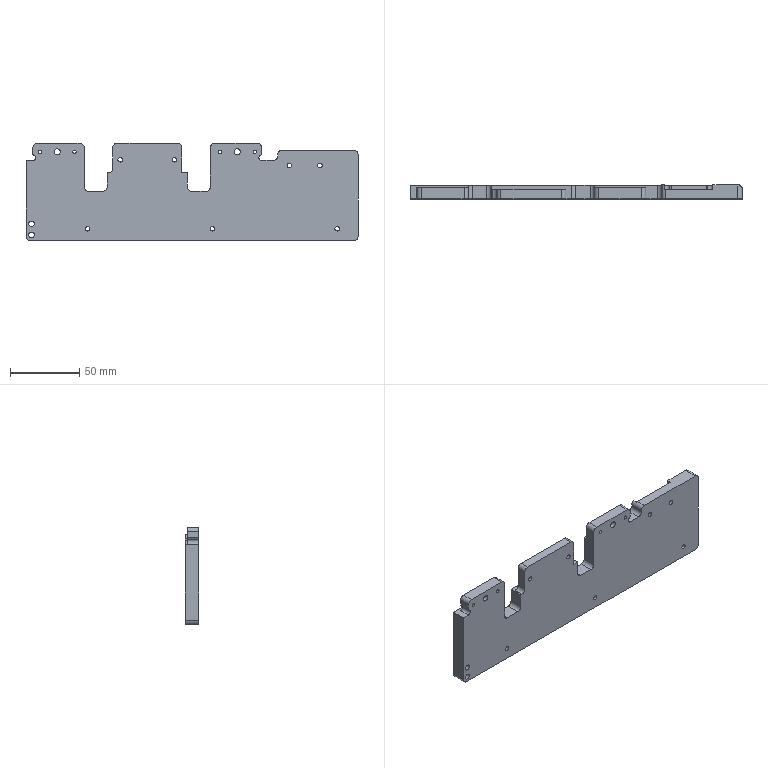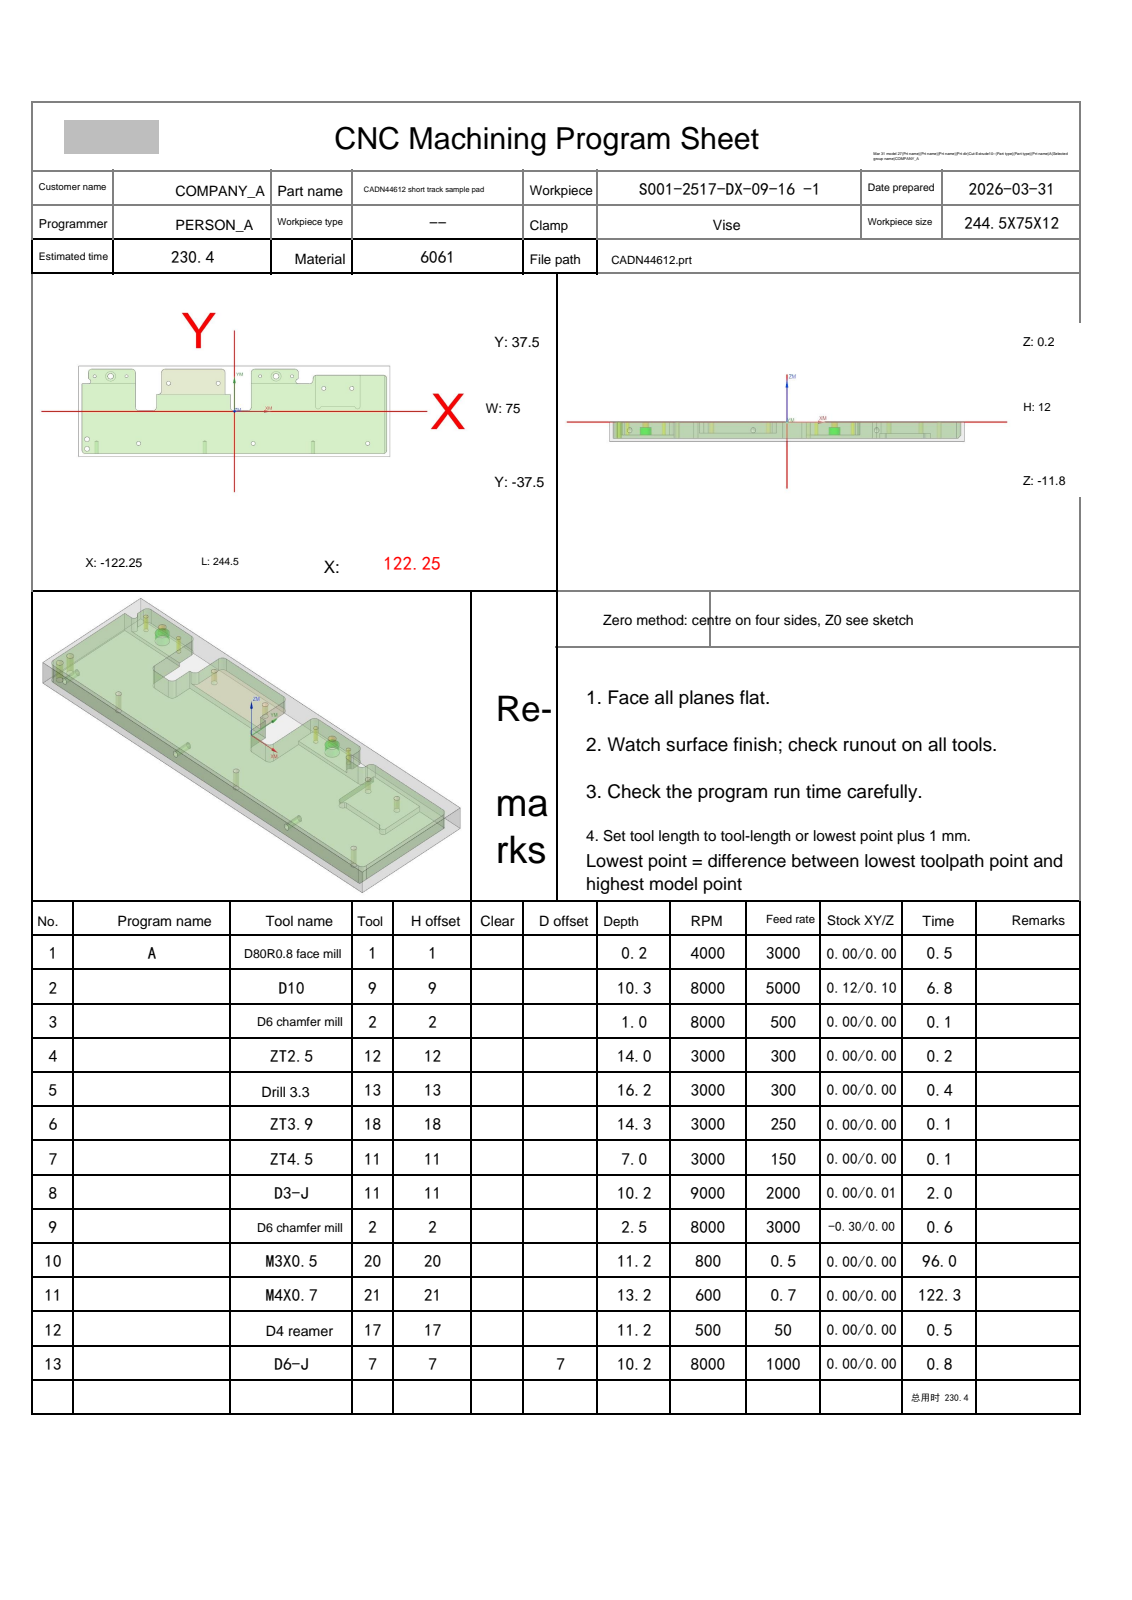NC program | NX | posted by the shop | part box 239.5 x 10 x 70 mm
Lines 10511 to 10745 of 10745:
N9 T02 M06
(D6 chamfer mill  D=6. R=0. H=02 ce=0.00 di=0.00)
G00 G90 G54 X.25 Y-37.128 M03 S8000
G43 H02 Z20.
M08
Z2.099
G01 Z-1.5 F3000.
G03 X.33 Y-36.828 I-.52 J.3
X.03 Y-36.308 I-.6 J0.0
G01 X0.0 Y-36.3
X-116.75
G02 X-121.05 Y-32. I0.0 J4.3
G01 Y22.8
G02 X-119.75 Y24.1 I1.3 J0.0
G01 X-114.75
G03 X-114.05 Y24.8 I0.0 J.7
X-114.176 Y25.2 I-.7 J0.0
G01 X-114.326 Y25.357
X-114.517 Y25.46
G02 X-116.05 Y27.628 I.767 J2.168
G01 Y32.
G02 X-111.75 Y36.3 I4.3 J0.0
G01 X-80.75
G02 X-76.45 Y32. I0.0 J-4.3
G01 Y3.5
G03 X-74.75 Y1.8 I1.7 J0.0
G01 X-64.25
G03 X-62.55 Y3.5 I0.0 J1.7
G01 Y14.
G02 X-61.25 Y15.3 I1.3 J0.0
G01 X-60.25
G03 X-58.55 Y17. I0.0 J1.7
G01 Y32.
G02 X-54.25 Y36.3 I4.3 J0.0
G01 X-10.25
G02 X-5.95 Y32. I0.0 J-4.3
G01 Y15.3
X-3.25
G02 X-1.95 Y14. I0.0 J-1.3
G01 Y3.5
G03 X-.25 Y1.8 I1.7 J0.0
G01 X10.25
G03 X11.95 Y3.5 I0.0 J1.7
G01 Y32.
G02 X16.25 Y36.3 I4.3 J0.0
G01 X47.25
G02 X51.55 Y32. I0.0 J-4.3
G01 Y27.628
G02 X50.017 Y25.46 I-2.3 J0.0
G03 X49.55 Y24.8 I.233 J-.66
X49.842 Y24.231 I.7 J0.0
G01 X50.036 Y24.134
X50.25 Y24.1
X58.75
G03 X60.45 Y25.8 I0.0 J1.7
G01 Y27.
G02 X64.75 Y31.3 I4.3 J0.0
G01 X116.75
G02 X121.05 Y27. I0.0 J-4.3
G01 Y-32.
G02 X116.75 Y-36.3 I-4.3 J0.0
G01 X0.0
X-.03 Y-36.308
G03 X-.33 Y-36.828 I.3 J-.52
X-.25 Y-37.128 I.6 J0.0
G01 Z2.099
G00 Z20.
G00 G90 X45.25 Y29. M03 S8000
Z20.
G98 G81 X45.25 Y29. Z-1.75 R3. F500.
X20.25
X-84.75
X-109.75
G80
G00 Z20.
G00 G90 X104.75 Y-26.5 M03 S8000
Z20.
G98 G81 X104.75 Y-26.5 Z-2.2 R3. F500.
X92.25 Y19.
X70.25
X14.75 Y-26.5
X-12.75 Y23.25
X-51.75
X-75.25 Y-26.5
G80
G00 Z20.
G00 G90 X-115.75 Y-23. M03 S8000
Z20.
G98 G81 X-115.75 Y-23. Z-2.3 R3. F500.
Y-31.
G80
G00 Z20.
G00 G90 X32.2 Y28.982 M03 S8000
Z20.
Z-.5
G01 Z-1. F500.
X31.25 Y28.95
G03 X32.75 Y27.45 I1.5 J0.0
X34.3 Y29. I0.0 J1.55
X32.75 Y30.55 I-1.55 J0.0
X31.2 Y29. I0.0 J-1.55
X32.75 Y27.45 I1.55 J0.0
X34.25 Y28.95 I0.0 J1.5
G01 X33.3 Y28.982
Z-.5
G00 Z20.
X-97.8
Z-.5
G01 Z-1.
X-98.75 Y28.95
G03 X-97.25 Y27.45 I1.5 J0.0
X-95.7 Y29. I0.0 J1.55
X-97.25 Y30.55 I-1.55 J0.0
X-98.8 Y29. I0.0 J-1.55
X-97.25 Y27.45 I1.55 J0.0
X-95.75 Y28.95 I0.0 J1.5
G01 X-96.7 Y28.982
Z-.5
G00 Z20.
G91 G28 Z0.0
M05
M09
G91 G28 Z0.0
M01
N10 T20 M06
(M3X0.5 D=2.5 DR_a=180 H=20)
G00 G90 G54 X45.25 Y29. M03 S800
G43 H20 Z20.
M08
G95
G98 G84 X45.25 Y29. Z-11. R1. F.5 Q5.
X20.25
X-84.75
X-109.75
G80
G94
G00 Z20.
G91 G28 Z0.0
M05
M09
G91 G28 Z0.0
M01
N11 T21 M06
(M4X0.7 D=3.3 DR_a=180 H=21)
G00 G90 G54 X104.75 Y-26.5 M03 S600
G43 H21 Z20.
M08
G95
G98 G84 X104.75 Y-26.5 Z-13. R1. F.7 Q4.
G98 G84 X92.25 Y19. Z-10. R1.
X70.25
G98 G84 X14.75 Y-26.5 Z-13. R1.
G98 G84 X-12.75 Y23.25 Z-9.8 R1.
X-51.75
G98 G84 X-75.25 Y-26.5 Z-13. R1.
G80
G94
G00 Z20.
G91 G28 Z0.0
M05
M09
G91 G28 Z0.0
M01
N12 T17 M06
(D4 reamer D=4. DR_a=180 H=17)
G00 G90 G54 X-115.75 Y-23. M03 S500
G43 H17 Z20.
M08
G98 G81 X-115.75 Y-23. Z-11. R1. F50.
Y-31.
G80
G00 Z20.
G91 G28 Z0.0
M05
M09
G91 G28 Z0.0
M01
N13 T07 M06
(D6-J  D=6. R=0. H=07 ce=0.00 di=0.00)
G00 G90 G54 X117.762 Y-39.128 M03 S8000
G43 H07 Z20.
M08
Z-9.5
G01 Z-10. F1000.
G41 D07
X117.747 Y-38.929
G03 X116.75 Y-38. I-.997 J-.071
G01 X-116.75
G02 X-122.75 Y-32. I0.0 J6.
G01 Y22.8
G02 X-119.75 Y25.8 I3. J0.0
G01 X-117.308
G02 X-117.75 Y27.628 I3.558 J1.828
G01 Y32.
G02 X-111.75 Y38. I6. J0.0
G01 X-80.75
G02 X-74.75 Y32. I0.0 J-6.
G01 Y3.5
X-64.25
Y14.
G02 X-61.25 Y17. I3. J0.0
G01 X-60.25
Y32.
G02 X-54.25 Y38. I6. J0.0
G01 X-10.25
G02 X-4.25 Y32. I0.0 J-6.
G01 Y17.
X-3.25
G02 X-.25 Y14. I0.0 J-3.
G01 Y3.5
X10.25
Y32.
G02 X16.25 Y38. I6. J0.0
G01 X47.25
G02 X53.25 Y32. I0.0 J-6.
G01 Y27.628
G02 X52.808 Y25.8 I-4. J0.0
G01 X58.75
Y27.
G02 X64.75 Y33. I6. J0.0
G01 X116.75
G02 X122.75 Y27. I0.0 J-6.
G01 Y-32.
G02 X116.75 Y-38. I-6. J0.0
G01 X116.25
G03 X115.25 Y-39. I0.0 J-1.
G01 G40 Y-39.2
Z-9.5
G00 Z20.
M05
M09
G91 G28 Z0.0
G91 G28 Y0.0
M30
%